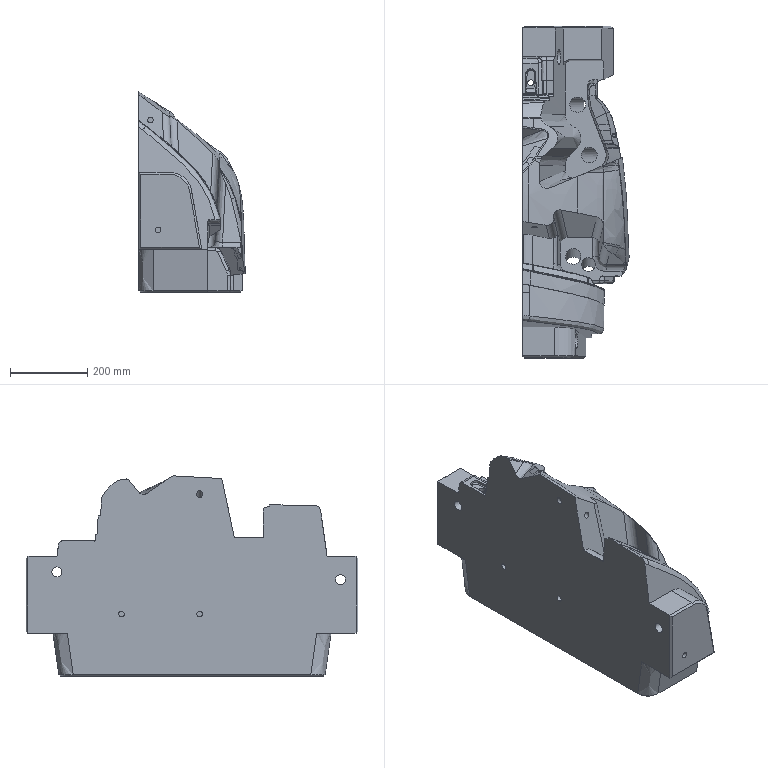Part | STEP file | solid 62 | 1 solid | 440 faces | box 275.804 x 860 x 518.917 mm | volume 54217917 mm3 | spline 276 | plane 78 | cylinder 64 | other 10 | cone 10 | sphere 2 | commonest cylinder face diameters 15 x21 26 x14 38 x6 21 x4 40 x3 70 x3